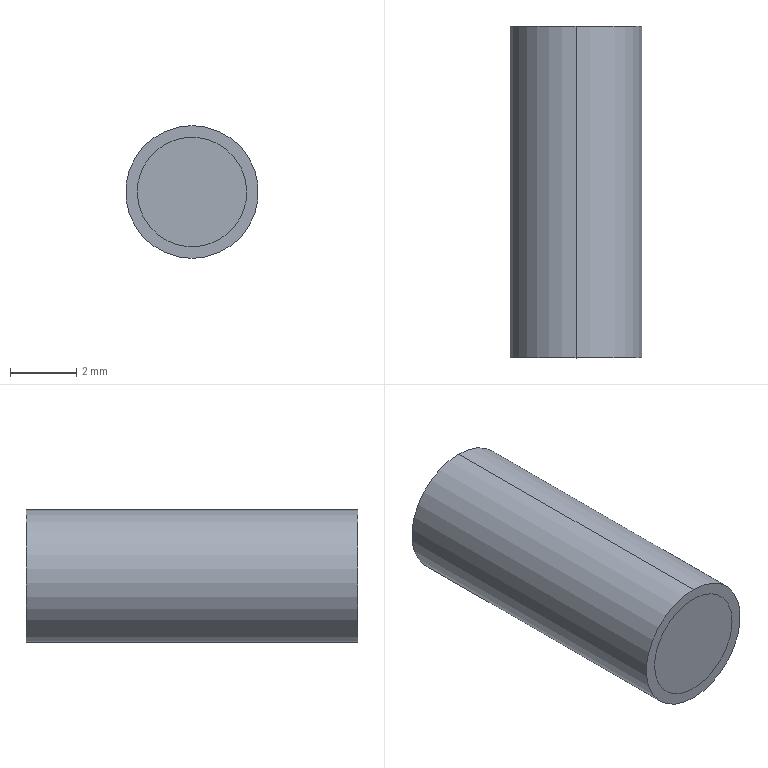Part | STEP file | 1 solid | 5 faces | box 4 x 10 x 4 mm | volume 125.664 mm3 | plane 3 | cylinder 2 | commonest cylinder face diameters 4 x2
STEP:
#1=CARTESIAN_POINT('',(0.,0.,0.));
#2=DIRECTION('',(0.,0.,1.));
#3=DIRECTION('',(1.,0.,0.));
#4=AXIS2_PLACEMENT_3D('',#1,#2,#3);
#5=CARTESIAN_POINT('',(-27.125,0.,-26.423));
#6=VERTEX_POINT('',#5);
#7=CARTESIAN_POINT('',(-27.125,0.,-22.423));
#8=VERTEX_POINT('',#7);
#9=CARTESIAN_POINT('',(-27.125,0.,-24.423));
#10=DIRECTION('',(0.,-1.,0.));
#11=DIRECTION('',(0.,0.,1.));
#12=AXIS2_PLACEMENT_3D('',#9,#10,#11);
#13=CIRCLE('',#12,2.);
#14=CARTESIAN_POINT('',(-27.125,0.,-24.423));
#15=DIRECTION('',(0.,1.,0.));
#16=DIRECTION('',(0.,0.,1.));
#17=AXIS2_PLACEMENT_3D('',#14,#15,#16);
#18=CYLINDRICAL_SURFACE('',#17,2.);
#19=CARTESIAN_POINT('',(6.283,0.));
#20=DIRECTION('',(-1.,0.));
#21=VECTOR('',#20,1.);
#22=LINE('',#19,#21);
#23=(GEOMETRIC_REPRESENTATION_CONTEXT(2)PARAMETRIC_REPRESENTATION_CONTEXT()REPRESENTATION_CONTEXT('',''));
#24=DEFINITIONAL_REPRESENTATION('',(#22),#23);
#25=PCURVE('',#18,#24);
#26=CARTESIAN_POINT('',(-24.957,0.,-26.591));
#27=DIRECTION('',(0.,1.,0.));
#28=DIRECTION('',(-1.,0.,0.));
#29=AXIS2_PLACEMENT_3D('',#26,#27,#28);
#30=PLANE('',#29);
#31=CARTESIAN_POINT('',(2.168,4.168));
#32=CARTESIAN_POINT('',(5.632,4.168));
#33=CARTESIAN_POINT('',(3.9,1.168));
#34=CARTESIAN_POINT('',(2.168,-1.832));
#35=CARTESIAN_POINT('',(0.436,1.168));
#36=CARTESIAN_POINT('',(-1.296,4.168));
#37=CARTESIAN_POINT('',(2.168,4.168));
#38=(BOUNDED_CURVE()B_SPLINE_CURVE(2,(#31,#32,#33,#34,#35,#36,#37),.UNSPECIFIED.,.T.,.F.)B_SPLINE_CURVE_WITH_KNOTS((1,2,2,2,2,1),(-2.094,0.,2.094,4.189,6.283,8.378),.UNSPECIFIED.)CURVE()GEOMETRIC_REPRESENTATION_ITEM()RATIONAL_B_SPLINE_CURVE((1.,0.5,1.,0.5,1.,0.5,1.))REPRESENTATION_ITEM(''));
#39=(GEOMETRIC_REPRESENTATION_CONTEXT(2)PARAMETRIC_REPRESENTATION_CONTEXT()REPRESENTATION_CONTEXT('',''));
#40=DEFINITIONAL_REPRESENTATION('',(#38),#39);
#41=PCURVE('',#30,#40);
#42=SURFACE_CURVE('',#13,(#25,#41),.PCURVE_S1.);
#43=EDGE_CURVE('',#6,#8,#42,.T.);
#44=ORIENTED_EDGE('',*,*,#43,.F.);
#45=CARTESIAN_POINT('',(-27.125,10.,-26.423));
#46=VERTEX_POINT('',#45);
#47=CARTESIAN_POINT('',(-27.125,0.,-26.423));
#48=DIRECTION('',(0.,1.,0.));
#49=VECTOR('',#48,1.);
#50=LINE('',#47,#49);
#51=CARTESIAN_POINT('',(3.142,0.));
#52=DIRECTION('',(0.,1.));
#53=VECTOR('',#52,1.);
#54=LINE('',#51,#53);
#55=(GEOMETRIC_REPRESENTATION_CONTEXT(2)PARAMETRIC_REPRESENTATION_CONTEXT()REPRESENTATION_CONTEXT('',''));
#56=DEFINITIONAL_REPRESENTATION('',(#54),#55);
#57=PCURVE('',#18,#56);
#58=CARTESIAN_POINT('',(-27.125,0.,-24.423));
#59=DIRECTION('',(0.,1.,0.));
#60=DIRECTION('',(0.,0.,1.));
#61=AXIS2_PLACEMENT_3D('',#58,#59,#60);
#62=CYLINDRICAL_SURFACE('',#61,2.);
#63=CARTESIAN_POINT('',(3.142,0.));
#64=DIRECTION('',(0.,1.));
#65=VECTOR('',#64,1.);
#66=LINE('',#63,#65);
#67=(GEOMETRIC_REPRESENTATION_CONTEXT(2)PARAMETRIC_REPRESENTATION_CONTEXT()REPRESENTATION_CONTEXT('',''));
#68=DEFINITIONAL_REPRESENTATION('',(#66),#67);
#69=PCURVE('',#62,#68);
#70=SURFACE_CURVE('',#50,(#57,#69),.PCURVE_S1.);
#71=EDGE_CURVE('',#6,#46,#70,.T.);
#72=ORIENTED_EDGE('',*,*,#71,.T.);
#73=CARTESIAN_POINT('',(-27.125,10.,-22.423));
#74=VERTEX_POINT('',#73);
#75=CARTESIAN_POINT('',(-27.125,10.,-24.423));
#76=DIRECTION('',(0.,1.,0.));
#77=DIRECTION('',(-1.,0.,0.));
#78=AXIS2_PLACEMENT_3D('',#75,#76,#77);
#79=CIRCLE('',#78,2.);
#80=CARTESIAN_POINT('',(-1.571,10.));
#81=DIRECTION('',(1.,0.));
#82=VECTOR('',#81,1.);
#83=LINE('',#80,#82);
#84=(GEOMETRIC_REPRESENTATION_CONTEXT(2)PARAMETRIC_REPRESENTATION_CONTEXT()REPRESENTATION_CONTEXT('',''));
#85=DEFINITIONAL_REPRESENTATION('',(#83),#84);
#86=PCURVE('',#18,#85);
#87=CARTESIAN_POINT('',(0.,10.,0.));
#88=DIRECTION('',(0.,-1.,0.));
#89=DIRECTION('',(0.,0.,-1.));
#90=AXIS2_PLACEMENT_3D('',#87,#88,#89);
#91=PLANE('',#90);
#92=CARTESIAN_POINT('',(24.423,-29.125));
#93=CARTESIAN_POINT('',(20.959,-29.125));
#94=CARTESIAN_POINT('',(22.691,-26.125));
#95=CARTESIAN_POINT('',(24.423,-23.125));
#96=CARTESIAN_POINT('',(26.155,-26.125));
#97=CARTESIAN_POINT('',(27.887,-29.125));
#98=CARTESIAN_POINT('',(24.423,-29.125));
#99=(BOUNDED_CURVE()B_SPLINE_CURVE(2,(#92,#93,#94,#95,#96,#97,#98),.UNSPECIFIED.,.T.,.F.)B_SPLINE_CURVE_WITH_KNOTS((1,2,2,2,2,1),(-2.094,0.,2.094,4.189,6.283,8.378),.UNSPECIFIED.)CURVE()GEOMETRIC_REPRESENTATION_ITEM()RATIONAL_B_SPLINE_CURVE((1.,0.5,1.,0.5,1.,0.5,1.))REPRESENTATION_ITEM(''));
#100=(GEOMETRIC_REPRESENTATION_CONTEXT(2)PARAMETRIC_REPRESENTATION_CONTEXT()REPRESENTATION_CONTEXT('',''));
#101=DEFINITIONAL_REPRESENTATION('',(#99),#100);
#102=PCURVE('',#91,#101);
#103=SURFACE_CURVE('',#79,(#86,#102),.PCURVE_S1.);
#104=EDGE_CURVE('',#74,#46,#103,.T.);
#105=ORIENTED_EDGE('',*,*,#104,.F.);
#106=CARTESIAN_POINT('',(-27.125,0.,-22.423));
#107=DIRECTION('',(0.,1.,0.));
#108=VECTOR('',#107,1.);
#109=LINE('',#106,#108);
#110=CARTESIAN_POINT('',(0.,0.));
#111=DIRECTION('',(0.,1.));
#112=VECTOR('',#111,1.);
#113=LINE('',#110,#112);
#114=(GEOMETRIC_REPRESENTATION_CONTEXT(2)PARAMETRIC_REPRESENTATION_CONTEXT()REPRESENTATION_CONTEXT('',''));
#115=DEFINITIONAL_REPRESENTATION('',(#113),#114);
#116=PCURVE('',#18,#115);
#117=CARTESIAN_POINT('',(6.283,0.));
#118=DIRECTION('',(0.,1.));
#119=VECTOR('',#118,1.);
#120=LINE('',#117,#119);
#121=(GEOMETRIC_REPRESENTATION_CONTEXT(2)PARAMETRIC_REPRESENTATION_CONTEXT()REPRESENTATION_CONTEXT('',''));
#122=DEFINITIONAL_REPRESENTATION('',(#120),#121);
#123=PCURVE('',#62,#122);
#124=SURFACE_CURVE('',#109,(#116,#123),.PCURVE_S1.);
#125=EDGE_CURVE('',#8,#74,#124,.T.);
#126=ORIENTED_EDGE('',*,*,#125,.F.);
#127=EDGE_LOOP('',(#44,#72,#105,#126));
#128=FACE_BOUND('',#127,.T.);
#129=ADVANCED_FACE('',(#128),#18,.T.);
#130=CARTESIAN_POINT('',(-28.775,0.,-24.423));
#131=VERTEX_POINT('',#130);
#132=CARTESIAN_POINT('',(-25.475,0.,-24.423));
#133=VERTEX_POINT('',#132);
#134=CARTESIAN_POINT('',(-28.775,0.,-24.423));
#135=CARTESIAN_POINT('',(-28.776,0.,-24.639));
#136=CARTESIAN_POINT('',(-28.732,0.,-24.856));
#137=CARTESIAN_POINT('',(-28.566,0.,-25.254));
#138=CARTESIAN_POINT('',(-28.444,0.,-25.438));
#139=CARTESIAN_POINT('',(-28.139,0.,-25.742));
#140=CARTESIAN_POINT('',(-27.955,0.,-25.865));
#141=CARTESIAN_POINT('',(-27.557,0.,-26.03));
#142=CARTESIAN_POINT('',(-27.341,0.,-26.073));
#143=CARTESIAN_POINT('',(-26.909,0.,-26.073));
#144=CARTESIAN_POINT('',(-26.693,0.,-26.03));
#145=CARTESIAN_POINT('',(-26.294,0.,-25.865));
#146=CARTESIAN_POINT('',(-26.11,0.,-25.742));
#147=CARTESIAN_POINT('',(-25.806,0.,-25.438));
#148=CARTESIAN_POINT('',(-25.684,0.,-25.254));
#149=CARTESIAN_POINT('',(-25.517,0.,-24.855));
#150=CARTESIAN_POINT('',(-25.474,0.,-24.64));
#151=CARTESIAN_POINT('',(-25.475,0.,-24.423));
#152=B_SPLINE_CURVE_WITH_KNOTS('',3,(#134,#135,#136,#137,#138,#139,#140,#141,#142,#143,#144,#145,#146,#147,#148,#149,#150,#151),.UNSPECIFIED.,.F.,.F.,(4,2,2,2,2,2,2,2,4),(0.,0.125,0.25,0.375,0.5,0.625,0.75,0.875,1.),.UNSPECIFIED.);
#153=CARTESIAN_POINT('',(-28.775,0.,-24.423));
#154=DIRECTION('',(0.,-1.,0.));
#155=DIRECTION('',(1.,0.,0.));
#156=AXIS2_PLACEMENT_3D('',#153,#154,#155);
#157=PLANE('',#156);
#158=CARTESIAN_POINT('',(0.,0.));
#159=CARTESIAN_POINT('',(-0.001239,-0.2156));
#160=CARTESIAN_POINT('',(0.04305,-0.4323));
#161=CARTESIAN_POINT('',(0.2084,-0.8304));
#162=CARTESIAN_POINT('',(0.3312,-1.014));
#163=CARTESIAN_POINT('',(0.6353,-1.319));
#164=CARTESIAN_POINT('',(0.8194,-1.442));
#165=CARTESIAN_POINT('',(1.218,-1.607));
#166=CARTESIAN_POINT('',(1.434,-1.65));
#167=CARTESIAN_POINT('',(1.866,-1.65));
#168=CARTESIAN_POINT('',(2.082,-1.607));
#169=CARTESIAN_POINT('',(2.481,-1.442));
#170=CARTESIAN_POINT('',(2.665,-1.319));
#171=CARTESIAN_POINT('',(2.969,-1.015));
#172=CARTESIAN_POINT('',(3.091,-0.831));
#173=CARTESIAN_POINT('',(3.257,-0.4317));
#174=CARTESIAN_POINT('',(3.301,-0.217));
#175=CARTESIAN_POINT('',(3.3,0.));
#176=B_SPLINE_CURVE_WITH_KNOTS('',3,(#158,#159,#160,#161,#162,#163,#164,#165,#166,#167,#168,#169,#170,#171,#172,#173,#174,#175),.UNSPECIFIED.,.F.,.F.,(4,2,2,2,2,2,2,2,4),(0.,0.125,0.25,0.375,0.5,0.625,0.75,0.875,1.),.UNSPECIFIED.);
#177=(GEOMETRIC_REPRESENTATION_CONTEXT(2)PARAMETRIC_REPRESENTATION_CONTEXT()REPRESENTATION_CONTEXT('',''));
#178=DEFINITIONAL_REPRESENTATION('',(#176),#177);
#179=PCURVE('',#157,#178);
#180=CARTESIAN_POINT('',(3.818,2.168));
#181=CARTESIAN_POINT('',(3.819,1.952));
#182=CARTESIAN_POINT('',(3.775,1.736));
#183=CARTESIAN_POINT('',(3.61,1.338));
#184=CARTESIAN_POINT('',(3.487,1.154));
#185=CARTESIAN_POINT('',(3.183,0.8491));
#186=CARTESIAN_POINT('',(2.999,0.7263));
#187=CARTESIAN_POINT('',(2.6,0.5611));
#188=CARTESIAN_POINT('',(2.384,0.5182));
#189=CARTESIAN_POINT('',(1.952,0.5179));
#190=CARTESIAN_POINT('',(1.736,0.5613));
#191=CARTESIAN_POINT('',(1.337,0.726));
#192=CARTESIAN_POINT('',(1.153,0.8495));
#193=CARTESIAN_POINT('',(0.8492,1.153));
#194=CARTESIAN_POINT('',(0.7269,1.337));
#195=CARTESIAN_POINT('',(0.5605,1.736));
#196=CARTESIAN_POINT('',(0.5168,1.951));
#197=CARTESIAN_POINT('',(0.518,2.168));
#198=B_SPLINE_CURVE_WITH_KNOTS('',3,(#180,#181,#182,#183,#184,#185,#186,#187,#188,#189,#190,#191,#192,#193,#194,#195,#196,#197),.UNSPECIFIED.,.F.,.F.,(4,2,2,2,2,2,2,2,4),(0.,0.125,0.25,0.375,0.5,0.625,0.75,0.875,1.),.UNSPECIFIED.);
#199=(GEOMETRIC_REPRESENTATION_CONTEXT(2)PARAMETRIC_REPRESENTATION_CONTEXT()REPRESENTATION_CONTEXT('',''));
#200=DEFINITIONAL_REPRESENTATION('',(#198),#199);
#201=PCURVE('',#30,#200);
#202=SURFACE_CURVE('',#152,(#179,#201),.PCURVE_S1.);
#203=EDGE_CURVE('',#131,#133,#202,.T.);
#204=ORIENTED_EDGE('',*,*,#203,.T.);
#205=CARTESIAN_POINT('',(-25.475,0.,-24.423));
#206=CARTESIAN_POINT('',(-25.474,0.,-24.208));
#207=CARTESIAN_POINT('',(-25.518,0.,-23.991));
#208=CARTESIAN_POINT('',(-25.683,0.,-23.593));
#209=CARTESIAN_POINT('',(-25.806,0.,-23.409));
#210=CARTESIAN_POINT('',(-26.11,0.,-23.104));
#211=CARTESIAN_POINT('',(-26.294,0.,-22.982));
#212=CARTESIAN_POINT('',(-26.693,0.,-22.816));
#213=CARTESIAN_POINT('',(-26.909,0.,-22.773));
#214=CARTESIAN_POINT('',(-27.341,0.,-22.773));
#215=CARTESIAN_POINT('',(-27.557,0.,-22.817));
#216=CARTESIAN_POINT('',(-27.955,0.,-22.981));
#217=CARTESIAN_POINT('',(-28.139,0.,-23.105));
#218=CARTESIAN_POINT('',(-28.444,0.,-23.408));
#219=CARTESIAN_POINT('',(-28.566,0.,-23.592));
#220=CARTESIAN_POINT('',(-28.732,0.,-23.992));
#221=CARTESIAN_POINT('',(-28.776,0.,-24.206));
#222=CARTESIAN_POINT('',(-28.775,0.,-24.423));
#223=B_SPLINE_CURVE_WITH_KNOTS('',3,(#205,#206,#207,#208,#209,#210,#211,#212,#213,#214,#215,#216,#217,#218,#219,#220,#221,#222),.UNSPECIFIED.,.F.,.F.,(4,2,2,2,2,2,2,2,4),(0.,0.125,0.25,0.375,0.5,0.625,0.75,0.875,1.),.UNSPECIFIED.);
#224=CARTESIAN_POINT('',(3.3,0.));
#225=CARTESIAN_POINT('',(3.301,0.2156));
#226=CARTESIAN_POINT('',(3.257,0.4323));
#227=CARTESIAN_POINT('',(3.092,0.8304));
#228=CARTESIAN_POINT('',(2.969,1.014));
#229=CARTESIAN_POINT('',(2.665,1.319));
#230=CARTESIAN_POINT('',(2.481,1.442));
#231=CARTESIAN_POINT('',(2.082,1.607));
#232=CARTESIAN_POINT('',(1.866,1.65));
#233=CARTESIAN_POINT('',(1.434,1.65));
#234=CARTESIAN_POINT('',(1.218,1.607));
#235=CARTESIAN_POINT('',(0.8193,1.442));
#236=CARTESIAN_POINT('',(0.6353,1.319));
#237=CARTESIAN_POINT('',(0.3312,1.015));
#238=CARTESIAN_POINT('',(0.2089,0.831));
#239=CARTESIAN_POINT('',(0.04251,0.4317));
#240=CARTESIAN_POINT('',(-0.001248,0.217));
#241=CARTESIAN_POINT('',(0.,0.));
#242=B_SPLINE_CURVE_WITH_KNOTS('',3,(#224,#225,#226,#227,#228,#229,#230,#231,#232,#233,#234,#235,#236,#237,#238,#239,#240,#241),.UNSPECIFIED.,.F.,.F.,(4,2,2,2,2,2,2,2,4),(0.,0.125,0.25,0.375,0.5,0.625,0.75,0.875,1.),.UNSPECIFIED.);
#243=(GEOMETRIC_REPRESENTATION_CONTEXT(2)PARAMETRIC_REPRESENTATION_CONTEXT()REPRESENTATION_CONTEXT('',''));
#244=DEFINITIONAL_REPRESENTATION('',(#242),#243);
#245=PCURVE('',#157,#244);
#246=CARTESIAN_POINT('',(0.518,2.168));
#247=CARTESIAN_POINT('',(0.5168,2.384));
#248=CARTESIAN_POINT('',(0.5611,2.6));
#249=CARTESIAN_POINT('',(0.7264,2.998));
#250=CARTESIAN_POINT('',(0.8492,3.182));
#251=CARTESIAN_POINT('',(1.153,3.487));
#252=CARTESIAN_POINT('',(1.337,3.61));
#253=CARTESIAN_POINT('',(1.736,3.775));
#254=CARTESIAN_POINT('',(1.952,3.818));
#255=CARTESIAN_POINT('',(2.384,3.818));
#256=CARTESIAN_POINT('',(2.6,3.775));
#257=CARTESIAN_POINT('',(2.999,3.61));
#258=CARTESIAN_POINT('',(3.183,3.487));
#259=CARTESIAN_POINT('',(3.487,3.183));
#260=CARTESIAN_POINT('',(3.609,2.999));
#261=CARTESIAN_POINT('',(3.775,2.6));
#262=CARTESIAN_POINT('',(3.819,2.385));
#263=CARTESIAN_POINT('',(3.818,2.168));
#264=B_SPLINE_CURVE_WITH_KNOTS('',3,(#246,#247,#248,#249,#250,#251,#252,#253,#254,#255,#256,#257,#258,#259,#260,#261,#262,#263),.UNSPECIFIED.,.F.,.F.,(4,2,2,2,2,2,2,2,4),(0.,0.125,0.25,0.375,0.5,0.625,0.75,0.875,1.),.UNSPECIFIED.);
#265=(GEOMETRIC_REPRESENTATION_CONTEXT(2)PARAMETRIC_REPRESENTATION_CONTEXT()REPRESENTATION_CONTEXT('',''));
#266=DEFINITIONAL_REPRESENTATION('',(#264),#265);
#267=PCURVE('',#30,#266);
#268=SURFACE_CURVE('',#223,(#245,#267),.PCURVE_S1.);
#269=EDGE_CURVE('',#133,#131,#268,.T.);
#270=ORIENTED_EDGE('',*,*,#269,.T.);
#271=EDGE_LOOP('',(#204,#270));
#272=FACE_BOUND('',#271,.T.);
#273=ADVANCED_FACE('',(#272),#157,.T.);
#274=ORIENTED_EDGE('',*,*,#104,.T.);
#275=CARTESIAN_POINT('',(-27.125,10.,-24.423));
#276=DIRECTION('',(0.,1.,0.));
#277=DIRECTION('',(-1.,0.,0.));
#278=AXIS2_PLACEMENT_3D('',#275,#276,#277);
#279=CIRCLE('',#278,2.);
#280=CARTESIAN_POINT('',(24.423,-29.125));
#281=CARTESIAN_POINT('',(20.959,-29.125));
#282=CARTESIAN_POINT('',(22.691,-26.125));
#283=CARTESIAN_POINT('',(24.423,-23.125));
#284=CARTESIAN_POINT('',(26.155,-26.125));
#285=CARTESIAN_POINT('',(27.887,-29.125));
#286=CARTESIAN_POINT('',(24.423,-29.125));
#287=(BOUNDED_CURVE()B_SPLINE_CURVE(2,(#280,#281,#282,#283,#284,#285,#286),.UNSPECIFIED.,.T.,.F.)B_SPLINE_CURVE_WITH_KNOTS((1,2,2,2,2,1),(-2.094,0.,2.094,4.189,6.283,8.378),.UNSPECIFIED.)CURVE()GEOMETRIC_REPRESENTATION_ITEM()RATIONAL_B_SPLINE_CURVE((1.,0.5,1.,0.5,1.,0.5,1.))REPRESENTATION_ITEM(''));
#288=(GEOMETRIC_REPRESENTATION_CONTEXT(2)PARAMETRIC_REPRESENTATION_CONTEXT()REPRESENTATION_CONTEXT('',''));
#289=DEFINITIONAL_REPRESENTATION('',(#287),#288);
#290=PCURVE('',#91,#289);
#291=CARTESIAN_POINT('',(-1.571,10.));
#292=DIRECTION('',(1.,0.));
#293=VECTOR('',#292,1.);
#294=LINE('',#291,#293);
#295=(GEOMETRIC_REPRESENTATION_CONTEXT(2)PARAMETRIC_REPRESENTATION_CONTEXT()REPRESENTATION_CONTEXT('',''));
#296=DEFINITIONAL_REPRESENTATION('',(#294),#295);
#297=PCURVE('',#62,#296);
#298=SURFACE_CURVE('',#279,(#290,#297),.PCURVE_S1.);
#299=EDGE_CURVE('',#46,#74,#298,.T.);
#300=ORIENTED_EDGE('',*,*,#299,.T.);
#301=EDGE_LOOP('',(#274,#300));
#302=FACE_BOUND('',#301,.T.);
#303=ADVANCED_FACE('',(#302),#91,.F.);
#304=ORIENTED_EDGE('',*,*,#269,.F.);
#305=ORIENTED_EDGE('',*,*,#203,.F.);
#306=EDGE_LOOP('',(#304,#305));
#307=FACE_BOUND('',#306,.T.);
#308=CARTESIAN_POINT('',(-27.125,0.,-24.423));
#309=DIRECTION('',(0.,-1.,0.));
#310=DIRECTION('',(0.,0.,1.));
#311=AXIS2_PLACEMENT_3D('',#308,#309,#310);
#312=CIRCLE('',#311,2.);
#313=CARTESIAN_POINT('',(2.168,4.168));
#314=CARTESIAN_POINT('',(5.632,4.168));
#315=CARTESIAN_POINT('',(3.9,1.168));
#316=CARTESIAN_POINT('',(2.168,-1.832));
#317=CARTESIAN_POINT('',(0.436,1.168));
#318=CARTESIAN_POINT('',(-1.296,4.168));
#319=CARTESIAN_POINT('',(2.168,4.168));
#320=(BOUNDED_CURVE()B_SPLINE_CURVE(2,(#313,#314,#315,#316,#317,#318,#319),.UNSPECIFIED.,.T.,.F.)B_SPLINE_CURVE_WITH_KNOTS((1,2,2,2,2,1),(-2.094,0.,2.094,4.189,6.283,8.378),.UNSPECIFIED.)CURVE()GEOMETRIC_REPRESENTATION_ITEM()RATIONAL_B_SPLINE_CURVE((1.,0.5,1.,0.5,1.,0.5,1.))REPRESENTATION_ITEM(''));
#321=(GEOMETRIC_REPRESENTATION_CONTEXT(2)PARAMETRIC_REPRESENTATION_CONTEXT()REPRESENTATION_CONTEXT('',''));
#322=DEFINITIONAL_REPRESENTATION('',(#320),#321);
#323=PCURVE('',#30,#322);
#324=CARTESIAN_POINT('',(6.283,0.));
#325=DIRECTION('',(-1.,0.));
#326=VECTOR('',#325,1.);
#327=LINE('',#324,#326);
#328=(GEOMETRIC_REPRESENTATION_CONTEXT(2)PARAMETRIC_REPRESENTATION_CONTEXT()REPRESENTATION_CONTEXT('',''));
#329=DEFINITIONAL_REPRESENTATION('',(#327),#328);
#330=PCURVE('',#62,#329);
#331=SURFACE_CURVE('',#312,(#323,#330),.PCURVE_S1.);
#332=EDGE_CURVE('',#8,#6,#331,.T.);
#333=ORIENTED_EDGE('',*,*,#332,.T.);
#334=ORIENTED_EDGE('',*,*,#43,.T.);
#335=EDGE_LOOP('',(#333,#334));
#336=FACE_BOUND('',#335,.T.);
#337=ADVANCED_FACE('',(#307,#336),#30,.F.);
#338=ORIENTED_EDGE('',*,*,#71,.F.);
#339=ORIENTED_EDGE('',*,*,#332,.F.);
#340=ORIENTED_EDGE('',*,*,#125,.T.);
#341=ORIENTED_EDGE('',*,*,#299,.F.);
#342=EDGE_LOOP('',(#338,#339,#340,#341));
#343=FACE_BOUND('',#342,.T.);
#344=ADVANCED_FACE('',(#343),#62,.T.);
#345=CLOSED_SHELL('',(#129,#273,#303,#337,#344));
#346=MANIFOLD_SOLID_BREP('',#345);
#347=(LENGTH_UNIT()NAMED_UNIT(*)SI_UNIT(.MILLI.,.METRE.));
#348=UNCERTAINTY_MEASURE_WITH_UNIT(LENGTH_MEASURE(0.0000001),#347,'','');
#349=(NAMED_UNIT(*)PLANE_ANGLE_UNIT()SI_UNIT($,.RADIAN.));
#350=(NAMED_UNIT(*)SI_UNIT($,.STERADIAN.)SOLID_ANGLE_UNIT());
#351=(GEOMETRIC_REPRESENTATION_CONTEXT(3)GLOBAL_UNCERTAINTY_ASSIGNED_CONTEXT((#348))GLOBAL_UNIT_ASSIGNED_CONTEXT((#347,#349,#350))REPRESENTATION_CONTEXT('',''));
#352=ADVANCED_BREP_SHAPE_REPRESENTATION('',(#4,#346),#351);